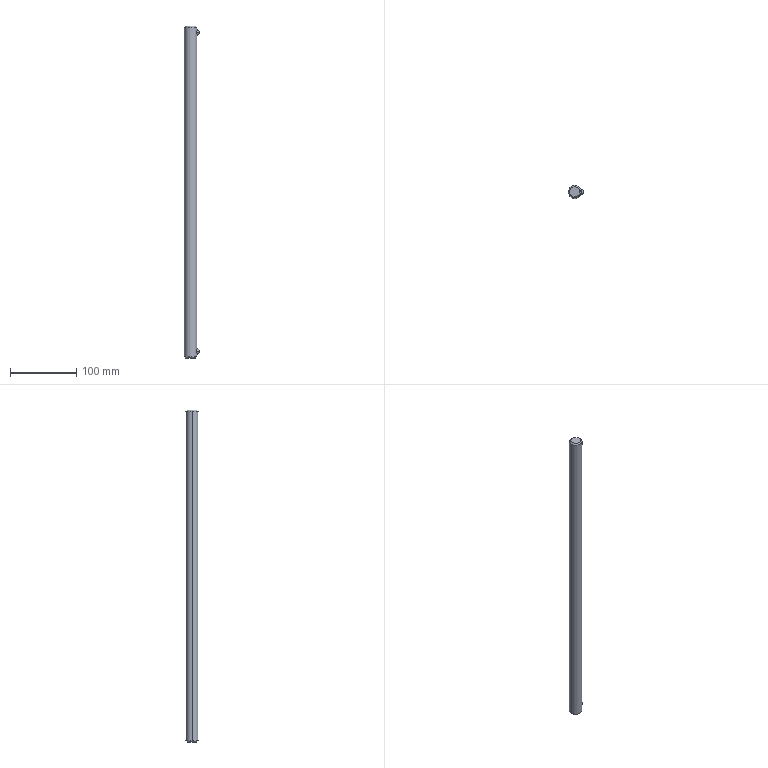Part | SolidWorks | features BaseBody 1 | 1 solid | 24 faces | box 23.05 x 19.05 x 500 mm | volume 142580 mm3 | spline 12 | cylinder 6 | cone 4 | plane 2 | commonest cylinder face diameters 8 x4 19.05 x2
STEP:
#1=CARTESIAN_POINT('',(22.554,-5.243,10.));
#2=VERTEX_POINT('',#1);
#3=CARTESIAN_POINT('',(18.554,-1.243,10.));
#4=VERTEX_POINT('',#3);
#5=CARTESIAN_POINT('',(18.554,-5.243,10.));
#6=DIRECTION('',(0.,0.,1.));
#7=DIRECTION('',(1.,0.,0.));
#8=AXIS2_PLACEMENT_3D('',#5,#6,#7);
#9=CIRCLE('',#8,4.);
#10=EDGE_CURVE('',#2,#4,#9,.T.);
#11=ORIENTED_EDGE('',*,*,#10,.F.);
#12=CARTESIAN_POINT('',(18.554,-9.243,10.));
#13=VERTEX_POINT('',#12);
#14=CARTESIAN_POINT('',(18.554,-5.243,10.));
#15=DIRECTION('',(0.,0.,-1.));
#16=DIRECTION('',(1.,0.,0.));
#17=AXIS2_PLACEMENT_3D('',#14,#15,#16);
#18=CIRCLE('',#17,4.);
#19=EDGE_CURVE('',#2,#13,#18,.T.);
#20=ORIENTED_EDGE('',*,*,#19,.T.);
#21=CARTESIAN_POINT('',(18.554,-8.022,7.123));
#22=VERTEX_POINT('',#21);
#23=CARTESIAN_POINT('',(18.554,-5.243,10.));
#24=DIRECTION('',(1.,0.,0.));
#25=DIRECTION('',(0.,1.,0.));
#26=AXIS2_PLACEMENT_3D('',#23,#24,#25);
#27=CIRCLE('',#26,4.);
#28=EDGE_CURVE('',#13,#22,#27,.T.);
#29=ORIENTED_EDGE('',*,*,#28,.T.);
#30=CARTESIAN_POINT('',(18.554,-2.464,7.123));
#31=VERTEX_POINT('',#30);
#32=CARTESIAN_POINT('',(18.554,-2.464,7.123));
#33=CARTESIAN_POINT('',(18.689,-2.875,6.725));
#34=CARTESIAN_POINT('',(18.951,-3.89,6.115));
#35=CARTESIAN_POINT('',(19.065,-6.011,5.891));
#36=CARTESIAN_POINT('',(18.757,-7.404,6.527));
#37=CARTESIAN_POINT('',(18.554,-8.022,7.123));
#38=B_SPLINE_CURVE_WITH_KNOTS('',3,(#32,#33,#34,#35,#36,#37),.UNSPECIFIED.,.F.,.F.,(4,1,1,4),(0.,0.2857,0.5714,1.),.UNSPECIFIED.);
#39=EDGE_CURVE('',#31,#22,#38,.T.);
#40=ORIENTED_EDGE('',*,*,#39,.F.);
#41=CARTESIAN_POINT('',(18.554,-5.243,10.));
#42=DIRECTION('',(1.,0.,0.));
#43=DIRECTION('',(0.,1.,0.));
#44=AXIS2_PLACEMENT_3D('',#41,#42,#43);
#45=CIRCLE('',#44,4.);
#46=EDGE_CURVE('',#31,#4,#45,.T.);
#47=ORIENTED_EDGE('',*,*,#46,.T.);
#48=EDGE_LOOP('',(#11,#20,#29,#40,#47));
#49=FACE_OUTER_BOUND('',#48,.T.);
#50=CARTESIAN_POINT('',(22.554,-5.243,10.));
#51=CARTESIAN_POINT('',(22.554,-5.243,10.));
#52=CARTESIAN_POINT('',(22.554,-5.243,10.));
#53=CARTESIAN_POINT('',(22.554,-5.243,10.));
#54=CARTESIAN_POINT('',(22.554,-7.586,10.));
#55=CARTESIAN_POINT('',(22.554,-7.586,5.314));
#56=CARTESIAN_POINT('',(22.554,-2.9,5.314));
#57=CARTESIAN_POINT('',(22.554,-2.9,10.));
#58=CARTESIAN_POINT('',(20.897,-9.243,10.));
#59=CARTESIAN_POINT('',(20.897,-9.243,2.));
#60=CARTESIAN_POINT('',(20.897,-1.243,2.));
#61=CARTESIAN_POINT('',(20.897,-1.243,10.));
#62=CARTESIAN_POINT('',(18.554,-9.243,10.));
#63=CARTESIAN_POINT('',(18.554,-9.243,2.));
#64=CARTESIAN_POINT('',(18.554,-1.243,2.));
#65=CARTESIAN_POINT('',(18.554,-1.243,10.));
#66=(BOUNDED_SURFACE()B_SPLINE_SURFACE(3,3,((#50,#51,#52,#53),(#54,#55,#56,#57),(#58,#59,#60,#61),(#62,#63,#64,#65)),.UNSPECIFIED.,.F.,.F.,.T.)B_SPLINE_SURFACE_WITH_KNOTS((4,4),(4,4),(0.,1.),(0.,1.),.UNSPECIFIED.)GEOMETRIC_REPRESENTATION_ITEM()RATIONAL_B_SPLINE_SURFACE(((1.,0.3333,0.3333,1.),(0.8047,0.2682,0.2682,0.8047),(0.8047,0.2682,0.2682,0.8047),(1.,0.3333,0.3333,1.)))REPRESENTATION_ITEM('')SURFACE());
#67=ADVANCED_FACE('',(#49),#66,.T.);
#68=CARTESIAN_POINT('',(22.554,-5.243,490.));
#69=VERTEX_POINT('',#68);
#70=CARTESIAN_POINT('',(18.554,-1.243,490.));
#71=VERTEX_POINT('',#70);
#72=CARTESIAN_POINT('',(18.554,-5.243,490.));
#73=DIRECTION('',(0.,0.,1.));
#74=DIRECTION('',(1.,0.,0.));
#75=AXIS2_PLACEMENT_3D('',#72,#73,#74);
#76=CIRCLE('',#75,4.);
#77=EDGE_CURVE('',#69,#71,#76,.T.);
#78=ORIENTED_EDGE('',*,*,#77,.F.);
#79=CARTESIAN_POINT('',(18.554,-9.243,490.));
#80=VERTEX_POINT('',#79);
#81=CARTESIAN_POINT('',(18.554,-5.243,490.));
#82=DIRECTION('',(0.,0.,-1.));
#83=DIRECTION('',(1.,0.,0.));
#84=AXIS2_PLACEMENT_3D('',#81,#82,#83);
#85=CIRCLE('',#84,4.);
#86=EDGE_CURVE('',#69,#80,#85,.T.);
#87=ORIENTED_EDGE('',*,*,#86,.T.);
#88=CARTESIAN_POINT('',(18.554,-8.022,487.123));
#89=VERTEX_POINT('',#88);
#90=CARTESIAN_POINT('',(18.554,-5.243,490.));
#91=DIRECTION('',(1.,0.,0.));
#92=DIRECTION('',(0.,1.,0.));
#93=AXIS2_PLACEMENT_3D('',#90,#91,#92);
#94=CIRCLE('',#93,4.);
#95=EDGE_CURVE('',#80,#89,#94,.T.);
#96=ORIENTED_EDGE('',*,*,#95,.T.);
#97=CARTESIAN_POINT('',(18.554,-2.464,487.123));
#98=VERTEX_POINT('',#97);
#99=CARTESIAN_POINT('',(18.554,-2.464,487.123));
#100=CARTESIAN_POINT('',(18.757,-3.081,486.527));
#101=CARTESIAN_POINT('',(19.067,-4.485,485.887));
#102=CARTESIAN_POINT('',(18.949,-6.602,486.119));
#103=CARTESIAN_POINT('',(18.689,-7.61,486.725));
#104=CARTESIAN_POINT('',(18.554,-8.022,487.123));
#105=B_SPLINE_CURVE_WITH_KNOTS('',3,(#99,#100,#101,#102,#103,#104),.UNSPECIFIED.,.F.,.F.,(4,1,1,4),(0.,0.4286,0.7143,1.),.UNSPECIFIED.);
#106=EDGE_CURVE('',#98,#89,#105,.T.);
#107=ORIENTED_EDGE('',*,*,#106,.F.);
#108=CARTESIAN_POINT('',(18.554,-5.243,490.));
#109=DIRECTION('',(1.,0.,0.));
#110=DIRECTION('',(0.,1.,0.));
#111=AXIS2_PLACEMENT_3D('',#108,#109,#110);
#112=CIRCLE('',#111,4.);
#113=EDGE_CURVE('',#98,#71,#112,.T.);
#114=ORIENTED_EDGE('',*,*,#113,.T.);
#115=EDGE_LOOP('',(#78,#87,#96,#107,#114));
#116=FACE_OUTER_BOUND('',#115,.T.);
#117=CARTESIAN_POINT('',(22.554,-5.243,490.));
#118=CARTESIAN_POINT('',(22.554,-5.243,490.));
#119=CARTESIAN_POINT('',(22.554,-5.243,490.));
#120=CARTESIAN_POINT('',(22.554,-5.243,490.));
#121=CARTESIAN_POINT('',(22.554,-7.586,490.));
#122=CARTESIAN_POINT('',(22.554,-7.586,485.314));
#123=CARTESIAN_POINT('',(22.554,-2.9,485.314));
#124=CARTESIAN_POINT('',(22.554,-2.9,490.));
#125=CARTESIAN_POINT('',(20.897,-9.243,490.));
#126=CARTESIAN_POINT('',(20.897,-9.243,482.));
#127=CARTESIAN_POINT('',(20.897,-1.243,482.));
#128=CARTESIAN_POINT('',(20.897,-1.243,490.));
#129=CARTESIAN_POINT('',(18.554,-9.243,490.));
#130=CARTESIAN_POINT('',(18.554,-9.243,482.));
#131=CARTESIAN_POINT('',(18.554,-1.243,482.));
#132=CARTESIAN_POINT('',(18.554,-1.243,490.));
#133=(BOUNDED_SURFACE()B_SPLINE_SURFACE(3,3,((#117,#118,#119,#120),(#121,#122,#123,#124),(#125,#126,#127,#128),(#129,#130,#131,#132)),.UNSPECIFIED.,.F.,.F.,.T.)B_SPLINE_SURFACE_WITH_KNOTS((4,4),(4,4),(0.,1.),(0.,1.),.UNSPECIFIED.)GEOMETRIC_REPRESENTATION_ITEM()RATIONAL_B_SPLINE_SURFACE(((1.,0.3333,0.3333,1.),(0.8047,0.2682,0.2682,0.8047),(0.8047,0.2682,0.2682,0.8047),(1.,0.3333,0.3333,1.)))REPRESENTATION_ITEM('')SURFACE());
#134=ADVANCED_FACE('',(#116),#133,.T.);
#135=CARTESIAN_POINT('',(18.554,-5.243,2.));
#136=VERTEX_POINT('',#135);
#137=CARTESIAN_POINT('',(-0.4959,-5.243,2.));
#138=VERTEX_POINT('',#137);
#139=CARTESIAN_POINT('',(9.029,-5.243,2.));
#140=DIRECTION('',(0.,0.,1.));
#141=DIRECTION('',(1.,0.,0.));
#142=AXIS2_PLACEMENT_3D('',#139,#140,#141);
#143=CIRCLE('',#142,9.525);
#144=EDGE_CURVE('',#136,#138,#143,.T.);
#145=ORIENTED_EDGE('',*,*,#144,.T.);
#146=CARTESIAN_POINT('',(-0.4959,-5.243,498.));
#147=VERTEX_POINT('',#146);
#148=CARTESIAN_POINT('',(-0.4959,-5.243,0.));
#149=DIRECTION('',(0.,0.,1.));
#150=VECTOR('',#149,1000.);
#151=LINE('',#148,#150);
#152=EDGE_CURVE('',#138,#147,#151,.T.);
#153=ORIENTED_EDGE('',*,*,#152,.T.);
#154=CARTESIAN_POINT('',(18.554,-5.243,498.));
#155=VERTEX_POINT('',#154);
#156=CARTESIAN_POINT('',(9.029,-5.243,498.));
#157=DIRECTION('',(0.,0.,-1.));
#158=DIRECTION('',(1.,0.,0.));
#159=AXIS2_PLACEMENT_3D('',#156,#157,#158);
#160=CIRCLE('',#159,9.525);
#161=EDGE_CURVE('',#147,#155,#160,.T.);
#162=ORIENTED_EDGE('',*,*,#161,.T.);
#163=CARTESIAN_POINT('',(18.554,-5.243,494.471));
#164=VERTEX_POINT('',#163);
#165=CARTESIAN_POINT('',(18.554,-5.243,0.));
#166=DIRECTION('',(0.,0.,1.));
#167=VECTOR('',#166,1000.);
#168=LINE('',#165,#167);
#169=EDGE_CURVE('',#164,#155,#168,.T.);
#170=ORIENTED_EDGE('',*,*,#169,.F.);
#171=CARTESIAN_POINT('',(18.079,-2.272,493.237));
#172=VERTEX_POINT('',#171);
#173=CARTESIAN_POINT('',(18.554,-5.243,494.471));
#174=CARTESIAN_POINT('',(18.554,-4.966,494.47));
#175=CARTESIAN_POINT('',(18.542,-4.689,494.443));
#176=CARTESIAN_POINT('',(18.494,-4.143,494.335));
#177=CARTESIAN_POINT('',(18.46,-3.88,494.255));
#178=CARTESIAN_POINT('',(18.372,-3.372,494.044));
#179=CARTESIAN_POINT('',(18.32,-3.131,493.915));
#180=CARTESIAN_POINT('',(18.205,-2.676,493.608));
#181=CARTESIAN_POINT('',(18.142,-2.465,493.432));
#182=CARTESIAN_POINT('',(18.079,-2.272,493.237));
#183=B_SPLINE_CURVE_WITH_KNOTS('',3,(#173,#174,#175,#176,#177,#178,#179,#180,#181,#182),.UNSPECIFIED.,.F.,.F.,(4,2,2,2,4),(0.4992,0.6244,0.7496,0.8748,1.),.UNSPECIFIED.);
#184=EDGE_CURVE('',#164,#172,#183,.T.);
#185=ORIENTED_EDGE('',*,*,#184,.T.);
#186=CARTESIAN_POINT('',(18.079,-2.272,486.763));
#187=VERTEX_POINT('',#186);
#188=CARTESIAN_POINT('',(18.079,-2.272,493.237));
#189=CARTESIAN_POINT('',(18.013,-2.069,493.03));
#190=CARTESIAN_POINT('',(17.946,-1.889,492.804));
#191=CARTESIAN_POINT('',(17.849,-1.645,492.429));
#192=CARTESIAN_POINT('',(17.818,-1.57,492.301));
#193=CARTESIAN_POINT('',(17.774,-1.467,492.104));
#194=CARTESIAN_POINT('',(17.753,-1.418,492.004));
#195=CARTESIAN_POINT('',(17.732,-1.372,491.902));
#196=CARTESIAN_POINT('',(17.719,-1.343,491.834));
#197=CARTESIAN_POINT('',(17.713,-1.329,491.801));
#198=CARTESIAN_POINT('',(17.653,-1.197,491.477));
#199=CARTESIAN_POINT('',(17.611,-1.111,491.185));
#200=CARTESIAN_POINT('',(17.555,-0.9959,490.595));
#201=CARTESIAN_POINT('',(17.541,-0.9679,490.299));
#202=CARTESIAN_POINT('',(17.542,-0.9692,489.843));
#203=CARTESIAN_POINT('',(17.545,-0.9767,489.692));
#204=CARTESIAN_POINT('',(17.56,-1.006,489.39));
#205=CARTESIAN_POINT('',(17.571,-1.029,489.237));
#206=CARTESIAN_POINT('',(17.6,-1.086,488.939));
#207=CARTESIAN_POINT('',(17.617,-1.122,488.793));
#208=CARTESIAN_POINT('',(17.647,-1.186,488.577));
#209=CARTESIAN_POINT('',(17.658,-1.209,488.506));
#210=CARTESIAN_POINT('',(17.681,-1.259,488.364));
#211=CARTESIAN_POINT('',(17.693,-1.286,488.293));
#212=CARTESIAN_POINT('',(17.731,-1.369,488.088));
#213=CARTESIAN_POINT('',(17.758,-1.431,487.955));
#214=CARTESIAN_POINT('',(17.802,-1.534,487.759));
#215=CARTESIAN_POINT('',(17.818,-1.57,487.694));
#216=CARTESIAN_POINT('',(17.849,-1.645,487.567));
#217=CARTESIAN_POINT('',(17.865,-1.685,487.502));
#218=CARTESIAN_POINT('',(17.945,-1.886,487.197));
#219=CARTESIAN_POINT('',(18.012,-2.068,486.971));
#220=CARTESIAN_POINT('',(18.079,-2.272,486.763));
#221=B_SPLINE_CURVE_WITH_KNOTS('',3,(#188,#189,#190,#191,#192,#193,#194,#195,#196,#197,#198,#199,#200,#201,#202,#203,#204,#205,#206,#207,#208,#209,#210,#211,#212,#213,#214,#215,#216,#217,#218,#219,#220),.UNSPECIFIED.,.F.,.F.,(4,2,2,1,2,2,2,2,2,2,2,2,2,2,2,2,4),(0.,0.125,0.1875,0.2187,0.2344,0.25,0.375,0.5,0.5625,0.625,0.6875,0.7187,0.75,0.8125,0.8437,0.875,1.),.UNSPECIFIED.);
#222=EDGE_CURVE('',#172,#187,#221,.T.);
#223=ORIENTED_EDGE('',*,*,#222,.T.);
#224=CARTESIAN_POINT('',(18.554,-5.243,485.529));
#225=VERTEX_POINT('',#224);
#226=CARTESIAN_POINT('',(18.079,-2.272,486.763));
#227=CARTESIAN_POINT('',(18.142,-2.463,486.569));
#228=CARTESIAN_POINT('',(18.204,-2.674,486.395));
#229=CARTESIAN_POINT('',(18.292,-3.02,486.163));
#230=CARTESIAN_POINT('',(18.319,-3.136,486.093));
#231=CARTESIAN_POINT('',(18.371,-3.378,485.964));
#232=CARTESIAN_POINT('',(18.395,-3.502,485.905));
#233=CARTESIAN_POINT('',(18.439,-3.758,485.799));
#234=CARTESIAN_POINT('',(18.459,-3.891,485.751));
#235=CARTESIAN_POINT('',(18.493,-4.155,485.67));
#236=CARTESIAN_POINT('',(18.507,-4.288,485.637));
#237=CARTESIAN_POINT('',(18.542,-4.692,485.556));
#238=CARTESIAN_POINT('',(18.554,-4.967,485.529));
#239=CARTESIAN_POINT('',(18.554,-5.243,485.529));
#240=B_SPLINE_CURVE_WITH_KNOTS('',3,(#226,#227,#228,#229,#230,#231,#232,#233,#234,#235,#236,#237,#238,#239),.UNSPECIFIED.,.F.,.F.,(4,2,2,2,2,2,4),(0.,0.1248,0.1872,0.2496,0.312,0.3744,0.4992),.UNSPECIFIED.);
#241=EDGE_CURVE('',#187,#225,#240,.T.);
#242=ORIENTED_EDGE('',*,*,#241,.T.);
#243=CARTESIAN_POINT('',(18.554,-5.243,14.471));
#244=VERTEX_POINT('',#243);
#245=CARTESIAN_POINT('',(18.554,-5.243,0.));
#246=DIRECTION('',(0.,0.,1.));
#247=VECTOR('',#246,1000.);
#248=LINE('',#245,#247);
#249=EDGE_CURVE('',#244,#225,#248,.T.);
#250=ORIENTED_EDGE('',*,*,#249,.F.);
#251=CARTESIAN_POINT('',(18.079,-2.272,13.237));
#252=VERTEX_POINT('',#251);
#253=CARTESIAN_POINT('',(18.554,-5.243,14.471));
#254=CARTESIAN_POINT('',(18.554,-5.105,14.471));
#255=CARTESIAN_POINT('',(18.551,-4.966,14.464));
#256=CARTESIAN_POINT('',(18.539,-4.69,14.437));
#257=CARTESIAN_POINT('',(18.53,-4.553,14.417));
#258=CARTESIAN_POINT('',(18.494,-4.143,14.335));
#259=CARTESIAN_POINT('',(18.46,-3.88,14.256));
#260=CARTESIAN_POINT('',(18.372,-3.372,14.045));
#261=CARTESIAN_POINT('',(18.32,-3.132,13.915));
#262=CARTESIAN_POINT('',(18.205,-2.676,13.608));
#263=CARTESIAN_POINT('',(18.142,-2.465,13.432));
#264=CARTESIAN_POINT('',(18.079,-2.272,13.237));
#265=B_SPLINE_CURVE_WITH_KNOTS('',3,(#253,#254,#255,#256,#257,#258,#259,#260,#261,#262,#263,#264),.UNSPECIFIED.,.F.,.F.,(4,2,2,2,2,4),(0.4992,0.5618,0.6244,0.7496,0.8748,1.),.UNSPECIFIED.);
#266=EDGE_CURVE('',#244,#252,#265,.T.);
#267=ORIENTED_EDGE('',*,*,#266,.T.);
#268=CARTESIAN_POINT('',(18.079,-2.272,6.763));
#269=VERTEX_POINT('',#268);
#270=CARTESIAN_POINT('',(18.079,-2.272,13.237));
#271=CARTESIAN_POINT('',(18.012,-2.069,13.03));
#272=CARTESIAN_POINT('',(17.946,-1.889,12.804));
#273=CARTESIAN_POINT('',(17.849,-1.645,12.43));
#274=CARTESIAN_POINT('',(17.818,-1.57,12.301));
#275=CARTESIAN_POINT('',(17.774,-1.467,12.104));
#276=CARTESIAN_POINT('',(17.753,-1.418,12.004));
#277=CARTESIAN_POINT('',(17.732,-1.372,11.902));
#278=CARTESIAN_POINT('',(17.719,-1.343,11.834));
#279=CARTESIAN_POINT('',(17.713,-1.329,11.801));
#280=CARTESIAN_POINT('',(17.653,-1.197,11.477));
#281=CARTESIAN_POINT('',(17.611,-1.11,11.186));
#282=CARTESIAN_POINT('',(17.555,-0.9955,10.596));
#283=CARTESIAN_POINT('',(17.541,-0.9675,10.299));
#284=CARTESIAN_POINT('',(17.541,-0.9687,9.844));
#285=CARTESIAN_POINT('',(17.545,-0.9763,9.693));
#286=CARTESIAN_POINT('',(17.56,-1.006,9.39));
#287=CARTESIAN_POINT('',(17.571,-1.028,9.238));
#288=CARTESIAN_POINT('',(17.599,-1.086,8.94));
#289=CARTESIAN_POINT('',(17.617,-1.122,8.794));
#290=CARTESIAN_POINT('',(17.647,-1.186,8.578));
#291=CARTESIAN_POINT('',(17.658,-1.209,8.506));
#292=CARTESIAN_POINT('',(17.681,-1.258,8.365));
#293=CARTESIAN_POINT('',(17.693,-1.285,8.293));
#294=CARTESIAN_POINT('',(17.731,-1.369,8.089));
#295=CARTESIAN_POINT('',(17.758,-1.431,7.955));
#296=CARTESIAN_POINT('',(17.802,-1.534,7.759));
#297=CARTESIAN_POINT('',(17.817,-1.57,7.695));
#298=CARTESIAN_POINT('',(17.849,-1.645,7.567));
#299=CARTESIAN_POINT('',(17.865,-1.685,7.503));
#300=CARTESIAN_POINT('',(17.945,-1.886,7.197));
#301=CARTESIAN_POINT('',(18.012,-2.068,6.971));
#302=CARTESIAN_POINT('',(18.079,-2.272,6.763));
#303=B_SPLINE_CURVE_WITH_KNOTS('',3,(#270,#271,#272,#273,#274,#275,#276,#277,#278,#279,#280,#281,#282,#283,#284,#285,#286,#287,#288,#289,#290,#291,#292,#293,#294,#295,#296,#297,#298,#299,#300,#301,#302),.UNSPECIFIED.,.F.,.F.,(4,2,2,1,2,2,2,2,2,2,2,2,2,2,2,2,4),(0.,0.125,0.1875,0.2187,0.2344,0.25,0.375,0.5,0.5625,0.625,0.6875,0.7187,0.75,0.8125,0.8437,0.875,1.),.UNSPECIFIED.);
#304=EDGE_CURVE('',#252,#269,#303,.T.);
#305=ORIENTED_EDGE('',*,*,#304,.T.);
#306=CARTESIAN_POINT('',(18.554,-5.243,5.53));
#307=VERTEX_POINT('',#306);
#308=CARTESIAN_POINT('',(18.079,-2.272,6.763));
#309=CARTESIAN_POINT('',(18.205,-2.656,6.373));
#310=CARTESIAN_POINT('',(18.329,-3.119,6.061));
#311=CARTESIAN_POINT('',(18.46,-3.881,5.744));
#312=CARTESIAN_POINT('',(18.495,-4.145,5.664));
#313=CARTESIAN_POINT('',(18.53,-4.554,5.584));
#314=CARTESIAN_POINT('',(18.539,-4.691,5.563));
#315=CARTESIAN_POINT('',(18.551,-4.966,5.537));
#316=CARTESIAN_POINT('',(18.554,-5.105,5.53));
#317=CARTESIAN_POINT('',(18.554,-5.243,5.53));
#318=B_SPLINE_CURVE_WITH_KNOTS('',3,(#308,#309,#310,#311,#312,#313,#314,#315,#316,#317),.UNSPECIFIED.,.F.,.F.,(4,2,2,2,4),(0.,0.2497,0.3746,0.437,0.4995),.UNSPECIFIED.);
#319=EDGE_CURVE('',#269,#307,#318,.T.);
#320=ORIENTED_EDGE('',*,*,#319,.T.);
#321=CARTESIAN_POINT('',(18.554,-5.243,0.));
#322=DIRECTION('',(0.,0.,1.));
#323=VECTOR('',#322,1000.);
#324=LINE('',#321,#323);
#325=EDGE_CURVE('',#136,#307,#324,.T.);
#326=ORIENTED_EDGE('',*,*,#325,.F.);
#327=EDGE_LOOP('',(#145,#153,#162,#170,#185,#223,#242,#250,#267,#305,#320,#326));
#328=FACE_OUTER_BOUND('',#327,.T.);
#329=CARTESIAN_POINT('',(9.029,-5.243,0.));
#330=DIRECTION('',(0.,0.,1.));
#331=DIRECTION('',(1.,0.,0.));
#332=AXIS2_PLACEMENT_3D('',#329,#330,#331);
#333=CYLINDRICAL_SURFACE('',#332,9.525);
#334=ADVANCED_FACE('',(#328),#333,.T.);
#335=CARTESIAN_POINT('',(1.504,-5.243,500.));
#336=VERTEX_POINT('',#335);
#337=CARTESIAN_POINT('',(16.554,-5.243,500.));
#338=VERTEX_POINT('',#337);
#339=CARTESIAN_POINT('',(9.029,-5.243,500.));
#340=DIRECTION('',(0.,0.,-1.));
#341=DIRECTION('',(-1.,0.,0.));
#342=AXIS2_PLACEMENT_3D('',#339,#340,#341);
#343=CIRCLE('',#342,7.525);
#344=EDGE_CURVE('',#336,#338,#343,.T.);
#345=ORIENTED_EDGE('',*,*,#344,.T.);
#346=CARTESIAN_POINT('',(18.554,-5.243,498.));
#347=DIRECTION('',(0.7071,0.,-0.7071));
#348=VECTOR('',#347,1000.);
#349=LINE('',#346,#348);
#350=EDGE_CURVE('',#338,#155,#349,.T.);
#351=ORIENTED_EDGE('',*,*,#350,.T.);
#352=ORIENTED_EDGE('',*,*,#161,.F.);
#353=CARTESIAN_POINT('',(-0.4959,-5.243,498.));
#354=DIRECTION('',(-0.7071,0.,-0.7071));
#355=VECTOR('',#354,1000.);
#356=LINE('',#353,#355);
#357=EDGE_CURVE('',#336,#147,#356,.T.);
#358=ORIENTED_EDGE('',*,*,#357,.F.);
#359=EDGE_LOOP('',(#345,#351,#352,#358));
#360=FACE_OUTER_BOUND('',#359,.T.);
#361=CARTESIAN_POINT('',(9.029,-5.243,498.));
#362=DIRECTION('',(0.,0.,-1.));
#363=DIRECTION('',(-1.,0.,0.));
#364=AXIS2_PLACEMENT_3D('',#361,#362,#363);
#365=CONICAL_SURFACE('',#364,9.525,0.7854);
#366=ADVANCED_FACE('',(#360),#365,.T.);
#367=CARTESIAN_POINT('',(16.554,-5.243,0.));
#368=VERTEX_POINT('',#367);
#369=CARTESIAN_POINT('',(1.504,-5.243,0.));
#370=VERTEX_POINT('',#369);
#371=CARTESIAN_POINT('',(9.029,-5.243,0.));
#372=DIRECTION('',(0.,0.,1.));
#373=DIRECTION('',(1.,0.,0.));
#374=AXIS2_PLACEMENT_3D('',#371,#372,#373);
#375=CIRCLE('',#374,7.525);
#376=EDGE_CURVE('',#368,#370,#375,.T.);
#377=ORIENTED_EDGE('',*,*,#376,.T.);
#378=CARTESIAN_POINT('',(-0.4959,-5.243,2.));
#379=DIRECTION('',(-0.7071,0.,0.7071));
#380=VECTOR('',#379,1000.);
#381=LINE('',#378,#380);
#382=EDGE_CURVE('',#370,#138,#381,.T.);
#383=ORIENTED_EDGE('',*,*,#382,.T.);
#384=ORIENTED_EDGE('',*,*,#144,.F.);
#385=CARTESIAN_POINT('',(18.554,-5.243,2.));
#386=DIRECTION('',(0.7071,0.,0.7071));
#387=VECTOR('',#386,1000.);
#388=LINE('',#385,#387);
#389=EDGE_CURVE('',#368,#136,#388,.T.);
#390=ORIENTED_EDGE('',*,*,#389,.F.);
#391=EDGE_LOOP('',(#377,#383,#384,#390));
#392=FACE_OUTER_BOUND('',#391,.T.);
#393=CARTESIAN_POINT('',(9.029,-5.243,2.));
#394=DIRECTION('',(0.,0.,1.));
#395=DIRECTION('',(1.,0.,0.));
#396=AXIS2_PLACEMENT_3D('',#393,#394,#395);
#397=CONICAL_SURFACE('',#396,9.525,0.7854);
#398=ADVANCED_FACE('',(#392),#397,.T.);
#399=ORIENTED_EDGE('',*,*,#152,.F.);
#400=CARTESIAN_POINT('',(9.029,-5.243,2.));
#401=DIRECTION('',(0.,0.,1.));
#402=DIRECTION('',(1.,0.,0.));
#403=AXIS2_PLACEMENT_3D('',#400,#401,#402);
#404=CIRCLE('',#403,9.525);
#405=EDGE_CURVE('',#138,#136,#404,.T.);
#406=ORIENTED_EDGE('',*,*,#405,.T.);
#407=ORIENTED_EDGE('',*,*,#325,.T.);
#408=CARTESIAN_POINT('',(18.079,-8.213,6.763));
#409=VERTEX_POINT('',#408);
#410=CARTESIAN_POINT('',(18.554,-5.243,5.53));
#411=CARTESIAN_POINT('',(18.554,-5.519,5.529));
#412=CARTESIAN_POINT('',(18.542,-5.795,5.556));
#413=CARTESIAN_POINT('',(18.495,-6.333,5.663));
#414=CARTESIAN_POINT('',(18.461,-6.597,5.744));
#415=CARTESIAN_POINT('',(18.394,-6.985,5.905));
#416=CARTESIAN_POINT('',(18.371,-7.108,5.963));
#417=CARTESIAN_POINT('',(18.319,-7.349,6.093));
#418=CARTESIAN_POINT('',(18.292,-7.467,6.163));
#419=CARTESIAN_POINT('',(18.234,-7.695,6.316));
#420=CARTESIAN_POINT('',(18.203,-7.806,6.399));
#421=CARTESIAN_POINT('',(18.142,-8.017,6.574));
#422=CARTESIAN_POINT('',(18.111,-8.117,6.666));
#423=CARTESIAN_POINT('',(18.079,-8.213,6.763));
#424=B_SPLINE_CURVE_WITH_KNOTS('',3,(#410,#411,#412,#413,#414,#415,#416,#417,#418,#419,#420,#421,#422,#423),.UNSPECIFIED.,.F.,.F.,(4,2,2,2,2,2,4),(0.4995,0.6246,0.7497,0.8123,0.8749,0.9374,1.),.UNSPECIFIED.);
#425=EDGE_CURVE('',#307,#409,#424,.T.);
#426=ORIENTED_EDGE('',*,*,#425,.T.);
#427=CARTESIAN_POINT('',(18.079,-8.213,13.237));
#428=VERTEX_POINT('',#427);
#429=CARTESIAN_POINT('',(18.079,-8.213,6.763));
#430=CARTESIAN_POINT('',(18.012,-8.416,6.97));
#431=CARTESIAN_POINT('',(17.946,-8.597,7.196));
#432=CARTESIAN_POINT('',(17.849,-8.841,7.57));
#433=CARTESIAN_POINT('',(17.818,-8.916,7.699));
#434=CARTESIAN_POINT('',(17.774,-9.019,7.896));
#435=CARTESIAN_POINT('',(17.753,-9.068,7.996));
#436=CARTESIAN_POINT('',(17.732,-9.113,8.098));
#437=CARTESIAN_POINT('',(17.719,-9.143,8.166));
#438=CARTESIAN_POINT('',(17.713,-9.157,8.199));
#439=CARTESIAN_POINT('',(17.653,-9.289,8.523));
#440=CARTESIAN_POINT('',(17.611,-9.375,8.814));
#441=CARTESIAN_POINT('',(17.555,-9.49,9.404));
#442=CARTESIAN_POINT('',(17.541,-9.518,9.701));
#443=CARTESIAN_POINT('',(17.541,-9.517,10.156));
#444=CARTESIAN_POINT('',(17.545,-9.509,10.307));
#445=CARTESIAN_POINT('',(17.56,-9.479,10.61));
#446=CARTESIAN_POINT('',(17.571,-9.457,10.762));
#447=CARTESIAN_POINT('',(17.599,-9.399,11.06));
#448=CARTESIAN_POINT('',(17.617,-9.364,11.207));
#449=CARTESIAN_POINT('',(17.647,-9.3,11.423));
#450=CARTESIAN_POINT('',(17.658,-9.277,11.494));
#451=CARTESIAN_POINT('',(17.681,-9.227,11.635));
#452=CARTESIAN_POINT('',(17.693,-9.2,11.707));
#453=CARTESIAN_POINT('',(17.731,-9.117,11.911));
#454=CARTESIAN_POINT('',(17.758,-9.055,12.045));
#455=CARTESIAN_POINT('',(17.802,-8.952,12.241));
#456=CARTESIAN_POINT('',(17.818,-8.916,12.305));
#457=CARTESIAN_POINT('',(17.849,-8.841,12.433));
#458=CARTESIAN_POINT('',(17.865,-8.8,12.498));
#459=CARTESIAN_POINT('',(17.945,-8.6,12.803));
#460=CARTESIAN_POINT('',(18.012,-8.418,13.029));
#461=CARTESIAN_POINT('',(18.079,-8.213,13.237));
#462=B_SPLINE_CURVE_WITH_KNOTS('',3,(#429,#430,#431,#432,#433,#434,#435,#436,#437,#438,#439,#440,#441,#442,#443,#444,#445,#446,#447,#448,#449,#450,#451,#452,#453,#454,#455,#456,#457,#458,#459,#460,#461),.UNSPECIFIED.,.F.,.F.,(4,2,2,1,2,2,2,2,2,2,2,2,2,2,2,2,4),(0.,0.125,0.1875,0.2188,0.2344,0.25,0.375,0.5,0.5625,0.625,0.6875,0.7187,0.75,0.8125,0.8437,0.875,1.),.UNSPECIFIED.);
#463=EDGE_CURVE('',#409,#428,#462,.T.);
#464=ORIENTED_EDGE('',*,*,#463,.T.);
#465=CARTESIAN_POINT('',(18.079,-8.213,13.237));
#466=CARTESIAN_POINT('',(18.142,-8.022,13.431));
#467=CARTESIAN_POINT('',(18.204,-7.812,13.605));
#468=CARTESIAN_POINT('',(18.292,-7.466,13.837));
#469=CARTESIAN_POINT('',(18.319,-7.349,13.907));
#470=CARTESIAN_POINT('',(18.371,-7.108,14.036));
#471=CARTESIAN_POINT('',(18.395,-6.983,14.095));
#472=CARTESIAN_POINT('',(18.439,-6.728,14.202));
#473=CARTESIAN_POINT('',(18.459,-6.595,14.249));
#474=CARTESIAN_POINT('',(18.493,-6.331,14.33));
#475=CARTESIAN_POINT('',(18.522,-6.064,14.397));
#476=CARTESIAN_POINT('',(18.539,-5.792,14.438));
#477=CARTESIAN_POINT('',(18.551,-5.519,14.464));
#478=CARTESIAN_POINT('',(18.554,-5.38,14.471));
#479=CARTESIAN_POINT('',(18.554,-5.243,14.471));
#480=B_SPLINE_CURVE_WITH_KNOTS('',3,(#465,#466,#467,#468,#469,#470,#471,#472,#473,#474,#475,#476,#477,#478,#479),.UNSPECIFIED.,.F.,.F.,(4,2,2,2,2,1,2,4),(0.,0.1248,0.1872,0.2496,0.312,0.3744,0.4368,0.4992),.UNSPECIFIED.);
#481=EDGE_CURVE('',#428,#244,#480,.T.);
#482=ORIENTED_EDGE('',*,*,#481,.T.);
#483=ORIENTED_EDGE('',*,*,#249,.T.);
#484=CARTESIAN_POINT('',(18.079,-8.213,486.763));
#485=VERTEX_POINT('',#484);
#486=CARTESIAN_POINT('',(18.554,-5.243,485.529));
#487=CARTESIAN_POINT('',(18.554,-5.519,485.53));
#488=CARTESIAN_POINT('',(18.542,-5.796,485.557));
#489=CARTESIAN_POINT('',(18.494,-6.342,485.665));
#490=CARTESIAN_POINT('',(18.46,-6.605,485.745));
#491=CARTESIAN_POINT('',(18.372,-7.113,485.956));
#492=CARTESIAN_POINT('',(18.32,-7.354,486.085));
#493=CARTESIAN_POINT('',(18.205,-7.81,486.392));
#494=CARTESIAN_POINT('',(18.142,-8.021,486.568));
#495=CARTESIAN_POINT('',(18.079,-8.213,486.763));
#496=B_SPLINE_CURVE_WITH_KNOTS('',3,(#486,#487,#488,#489,#490,#491,#492,#493,#494,#495),.UNSPECIFIED.,.F.,.F.,(4,2,2,2,4),(0.4992,0.6244,0.7496,0.8748,1.),.UNSPECIFIED.);
#497=EDGE_CURVE('',#225,#485,#496,.T.);
#498=ORIENTED_EDGE('',*,*,#497,.T.);
#499=CARTESIAN_POINT('',(18.079,-8.213,493.237));
#500=VERTEX_POINT('',#499);
#501=CARTESIAN_POINT('',(18.079,-8.213,486.763));
#502=CARTESIAN_POINT('',(18.013,-8.416,486.97));
#503=CARTESIAN_POINT('',(17.946,-8.597,487.196));
#504=CARTESIAN_POINT('',(17.849,-8.841,487.571));
#505=CARTESIAN_POINT('',(17.818,-8.915,487.699));
#506=CARTESIAN_POINT('',(17.774,-9.018,487.896));
#507=CARTESIAN_POINT('',(17.753,-9.067,487.996));
#508=CARTESIAN_POINT('',(17.732,-9.113,488.098));
#509=CARTESIAN_POINT('',(17.719,-9.143,488.166));
#510=CARTESIAN_POINT('',(17.713,-9.157,488.199));
#511=CARTESIAN_POINT('',(17.653,-9.288,488.523));
#512=CARTESIAN_POINT('',(17.611,-9.375,488.815));
#513=CARTESIAN_POINT('',(17.555,-9.49,489.405));
#514=CARTESIAN_POINT('',(17.541,-9.518,489.701));
#515=CARTESIAN_POINT('',(17.542,-9.516,490.157));
#516=CARTESIAN_POINT('',(17.545,-9.509,490.308));
#517=CARTESIAN_POINT('',(17.56,-9.479,490.61));
#518=CARTESIAN_POINT('',(17.571,-9.457,490.763));
#519=CARTESIAN_POINT('',(17.6,-9.399,491.061));
#520=CARTESIAN_POINT('',(17.617,-9.363,491.207));
#521=CARTESIAN_POINT('',(17.647,-9.299,491.423));
#522=CARTESIAN_POINT('',(17.658,-9.276,491.494));
#523=CARTESIAN_POINT('',(17.681,-9.227,491.636));
#524=CARTESIAN_POINT('',(17.693,-9.2,491.707));
#525=CARTESIAN_POINT('',(17.731,-9.117,491.912));
#526=CARTESIAN_POINT('',(17.758,-9.055,492.045));
#527=CARTESIAN_POINT('',(17.802,-8.952,492.241));
#528=CARTESIAN_POINT('',(17.818,-8.916,492.306));
#529=CARTESIAN_POINT('',(17.849,-8.84,492.433));
#530=CARTESIAN_POINT('',(17.865,-8.8,492.498));
#531=CARTESIAN_POINT('',(17.945,-8.6,492.803));
#532=CARTESIAN_POINT('',(18.012,-8.418,493.029));
#533=CARTESIAN_POINT('',(18.079,-8.213,493.237));
#534=B_SPLINE_CURVE_WITH_KNOTS('',3,(#501,#502,#503,#504,#505,#506,#507,#508,#509,#510,#511,#512,#513,#514,#515,#516,#517,#518,#519,#520,#521,#522,#523,#524,#525,#526,#527,#528,#529,#530,#531,#532,#533),.UNSPECIFIED.,.F.,.F.,(4,2,2,1,2,2,2,2,2,2,2,2,2,2,2,2,4),(0.,0.125,0.1875,0.2188,0.2344,0.25,0.375,0.5,0.5625,0.625,0.6875,0.7188,0.75,0.8125,0.8438,0.875,1.),.UNSPECIFIED.);
#535=EDGE_CURVE('',#485,#500,#534,.T.);
#536=ORIENTED_EDGE('',*,*,#535,.T.);
#537=CARTESIAN_POINT('',(18.079,-8.213,493.237));
#538=CARTESIAN_POINT('',(18.142,-8.022,493.431));
#539=CARTESIAN_POINT('',(18.204,-7.812,493.605));
#540=CARTESIAN_POINT('',(18.292,-7.466,493.837));
#541=CARTESIAN_POINT('',(18.319,-7.349,493.907));
#542=CARTESIAN_POINT('',(18.371,-7.108,494.036));
#543=CARTESIAN_POINT('',(18.395,-6.983,494.095));
#544=CARTESIAN_POINT('',(18.439,-6.728,494.201));
#545=CARTESIAN_POINT('',(18.459,-6.595,494.249));
#546=CARTESIAN_POINT('',(18.493,-6.331,494.33));
#547=CARTESIAN_POINT('',(18.507,-6.197,494.363));
#548=CARTESIAN_POINT('',(18.542,-5.794,494.444));
#549=CARTESIAN_POINT('',(18.554,-5.518,494.471));
#550=CARTESIAN_POINT('',(18.554,-5.243,494.471));
#551=B_SPLINE_CURVE_WITH_KNOTS('',3,(#537,#538,#539,#540,#541,#542,#543,#544,#545,#546,#547,#548,#549,#550),.UNSPECIFIED.,.F.,.F.,(4,2,2,2,2,2,4),(0.,0.1248,0.1872,0.2496,0.312,0.3744,0.4992),.UNSPECIFIED.);
#552=EDGE_CURVE('',#500,#164,#551,.T.);
#553=ORIENTED_EDGE('',*,*,#552,.T.);
#554=ORIENTED_EDGE('',*,*,#169,.T.);
#555=CARTESIAN_POINT('',(9.029,-5.243,498.));
#556=DIRECTION('',(0.,0.,-1.));
#557=DIRECTION('',(1.,0.,0.));
#558=AXIS2_PLACEMENT_3D('',#555,#556,#557);
#559=CIRCLE('',#558,9.525);
#560=EDGE_CURVE('',#155,#147,#559,.T.);
#561=ORIENTED_EDGE('',*,*,#560,.T.);
#562=EDGE_LOOP('',(#399,#406,#407,#426,#464,#482,#483,#498,#536,#553,#554,#561));
#563=FACE_OUTER_BOUND('',#562,.T.);
#564=CARTESIAN_POINT('',(9.029,-5.243,0.));
#565=DIRECTION('',(0.,0.,1.));
#566=DIRECTION('',(1.,0.,0.));
#567=AXIS2_PLACEMENT_3D('',#564,#565,#566);
#568=CYLINDRICAL_SURFACE('',#567,9.525);
#569=ADVANCED_FACE('',(#563),#568,.T.);
#570=CARTESIAN_POINT('',(18.554,-8.022,12.877));
#571=VERTEX_POINT('',#570);
#572=CARTESIAN_POINT('',(18.079,-8.213,13.237));
#573=CARTESIAN_POINT('',(18.103,-8.141,13.153));
#574=CARTESIAN_POINT('',(18.226,-8.021,12.988));
#575=CARTESIAN_POINT('',(18.444,-8.003,12.895));
#576=CARTESIAN_POINT('',(18.554,-8.022,12.877));
#577=B_SPLINE_CURVE_WITH_KNOTS('',3,(#572,#573,#574,#575,#576),.UNSPECIFIED.,.F.,.F.,(4,1,4),(0.,0.5,1.),.UNSPECIFIED.);
#578=EDGE_CURVE('',#428,#571,#577,.T.);
#579=ORIENTED_EDGE('',*,*,#578,.T.);
#580=CARTESIAN_POINT('',(18.554,-2.464,12.877));
#581=VERTEX_POINT('',#580);
#582=CARTESIAN_POINT('',(18.554,-8.022,12.877));
#583=CARTESIAN_POINT('',(18.757,-7.404,13.473));
#584=CARTESIAN_POINT('',(19.067,-6.001,14.113));
#585=CARTESIAN_POINT('',(18.95,-3.883,13.882));
#586=CARTESIAN_POINT('',(18.689,-2.875,13.275));
#587=CARTESIAN_POINT('',(18.554,-2.464,12.877));
#588=B_SPLINE_CURVE_WITH_KNOTS('',3,(#582,#583,#584,#585,#586,#587),.UNSPECIFIED.,.F.,.F.,(4,1,1,4),(0.,0.4286,0.7143,1.),.UNSPECIFIED.);
#589=EDGE_CURVE('',#571,#581,#588,.T.);
#590=ORIENTED_EDGE('',*,*,#589,.T.);
#591=CARTESIAN_POINT('',(18.554,-2.464,12.877));
#592=CARTESIAN_POINT('',(18.444,-2.482,12.895));
#593=CARTESIAN_POINT('',(18.226,-2.464,12.988));
#594=CARTESIAN_POINT('',(18.103,-2.345,13.153));
#595=CARTESIAN_POINT('',(18.079,-2.272,13.237));
#596=B_SPLINE_CURVE_WITH_KNOTS('',3,(#591,#592,#593,#594,#595),.UNSPECIFIED.,.F.,.F.,(4,1,4),(0.,0.5,1.),.UNSPECIFIED.);
#597=EDGE_CURVE('',#581,#252,#596,.T.);
#598=ORIENTED_EDGE('',*,*,#597,.T.);
#599=ORIENTED_EDGE('',*,*,#266,.F.);
#600=ORIENTED_EDGE('',*,*,#481,.F.);
#601=EDGE_LOOP('',(#579,#590,#598,#599,#600));
#602=FACE_OUTER_BOUND('',#601,.T.);
#603=CARTESIAN_POINT('',(18.079,-8.213,13.237));
#604=CARTESIAN_POINT('',(18.296,-7.553,13.908));
#605=CARTESIAN_POINT('',(18.627,-6.053,14.627));
#606=CARTESIAN_POINT('',(18.502,-3.79,14.367));
#607=CARTESIAN_POINT('',(18.224,-2.712,13.684));
#608=CARTESIAN_POINT('',(18.079,-2.272,13.237));
#609=CARTESIAN_POINT('',(18.103,-8.141,13.153));
#610=CARTESIAN_POINT('',(18.309,-7.493,13.805));
#611=CARTESIAN_POINT('',(18.623,-6.03,14.5));
#612=CARTESIAN_POINT('',(18.505,-3.83,14.249));
#613=CARTESIAN_POINT('',(18.241,-2.776,13.588));
#614=CARTESIAN_POINT('',(18.103,-2.345,13.153));
#615=CARTESIAN_POINT('',(18.226,-8.021,12.988));
#616=CARTESIAN_POINT('',(18.42,-7.395,13.601));
#617=CARTESIAN_POINT('',(18.711,-5.993,14.247));
#618=CARTESIAN_POINT('',(18.601,-3.896,14.014));
#619=CARTESIAN_POINT('',(18.355,-2.882,13.397));
#620=CARTESIAN_POINT('',(18.226,-2.464,12.988));
#621=CARTESIAN_POINT('',(18.444,-8.003,12.895));
#622=CARTESIAN_POINT('',(18.643,-7.386,13.491));
#623=CARTESIAN_POINT('',(18.944,-5.991,14.125));
#624=CARTESIAN_POINT('',(18.83,-3.899,13.896));
#625=CARTESIAN_POINT('',(18.577,-2.894,13.293));
#626=CARTESIAN_POINT('',(18.444,-2.482,12.895));
#627=CARTESIAN_POINT('',(18.554,-8.022,12.877));
#628=CARTESIAN_POINT('',(18.757,-7.404,13.473));
#629=CARTESIAN_POINT('',(19.067,-6.001,14.113));
#630=CARTESIAN_POINT('',(18.95,-3.883,13.882));
#631=CARTESIAN_POINT('',(18.689,-2.875,13.275));
#632=CARTESIAN_POINT('',(18.554,-2.464,12.877));
#633=B_SPLINE_SURFACE_WITH_KNOTS('',3,3,((#603,#604,#605,#606,#607,#608),(#609,#610,#611,#612,#613,#614),(#615,#616,#617,#618,#619,#620),(#621,#622,#623,#624,#625,#626),(#627,#628,#629,#630,#631,#632)),.UNSPECIFIED.,.F.,.F.,.F.,(4,1,4),(4,1,1,4),(0.,0.5,1.),(-0.6947,-0.397,-0.1985,0.),.UNSPECIFIED.);
#634=ADVANCED_FACE('',(#602),#633,.T.);
#635=CARTESIAN_POINT('',(18.079,-8.213,6.763));
#636=CARTESIAN_POINT('',(18.103,-8.141,6.847));
#637=CARTESIAN_POINT('',(18.226,-8.021,7.012));
#638=CARTESIAN_POINT('',(18.444,-8.003,7.105));
#639=CARTESIAN_POINT('',(18.554,-8.022,7.123));
#640=B_SPLINE_CURVE_WITH_KNOTS('',3,(#635,#636,#637,#638,#639),.UNSPECIFIED.,.F.,.F.,(4,1,4),(0.,0.5,1.),.UNSPECIFIED.);
#641=EDGE_CURVE('',#409,#22,#640,.T.);
#642=ORIENTED_EDGE('',*,*,#641,.T.);
#643=CARTESIAN_POINT('',(18.554,-8.022,7.123));
#644=CARTESIAN_POINT('',(18.314,-8.671,7.75));
#645=CARTESIAN_POINT('',(17.892,-9.401,9.203));
#646=CARTESIAN_POINT('',(18.056,-9.135,11.422));
#647=CARTESIAN_POINT('',(18.394,-8.455,12.459));
#648=CARTESIAN_POINT('',(18.554,-8.022,12.877));
#649=B_SPLINE_CURVE_WITH_KNOTS('',3,(#643,#644,#645,#646,#647,#648),.UNSPECIFIED.,.F.,.F.,(4,1,1,4),(0.,0.4286,0.7143,1.),.UNSPECIFIED.);
#650=EDGE_CURVE('',#22,#571,#649,.T.);
#651=ORIENTED_EDGE('',*,*,#650,.T.);
#652=ORIENTED_EDGE('',*,*,#578,.F.);
#653=ORIENTED_EDGE('',*,*,#463,.F.);
#654=EDGE_LOOP('',(#642,#651,#652,#653));
#655=FACE_OUTER_BOUND('',#654,.T.);
#656=CARTESIAN_POINT('',(18.079,-8.213,6.763));
#657=CARTESIAN_POINT('',(17.851,-8.907,7.469));
#658=CARTESIAN_POINT('',(17.45,-9.687,9.104));
#659=CARTESIAN_POINT('',(17.606,-9.403,11.6));
#660=CARTESIAN_POINT('',(17.927,-8.676,12.766));
#661=CARTESIAN_POINT('',(18.079,-8.213,13.237));
#662=CARTESIAN_POINT('',(18.103,-8.141,6.847));
#663=CARTESIAN_POINT('',(17.885,-8.825,7.529));
#664=CARTESIAN_POINT('',(17.494,-9.605,9.123));
#665=CARTESIAN_POINT('',(17.646,-9.32,11.564));
#666=CARTESIAN_POINT('',(17.957,-8.597,12.698));
#667=CARTESIAN_POINT('',(18.103,-8.141,13.153));
#668=CARTESIAN_POINT('',(18.226,-8.021,7.012));
#669=CARTESIAN_POINT('',(18.012,-8.689,7.65));
#670=CARTESIAN_POINT('',(17.623,-9.463,9.162));
#671=CARTESIAN_POINT('',(17.774,-9.18,11.493));
#672=CARTESIAN_POINT('',(18.083,-8.466,12.562));
#673=CARTESIAN_POINT('',(18.226,-8.021,12.988));
#674=CARTESIAN_POINT('',(18.444,-8.003,7.105));
#675=CARTESIAN_POINT('',(18.213,-8.657,7.728));
#676=CARTESIAN_POINT('',(17.803,-9.405,9.192));
#677=CARTESIAN_POINT('',(17.962,-9.132,11.44));
#678=CARTESIAN_POINT('',(18.29,-8.439,12.479));
#679=CARTESIAN_POINT('',(18.444,-8.003,12.895));
#680=CARTESIAN_POINT('',(18.554,-8.022,7.123));
#681=CARTESIAN_POINT('',(18.314,-8.671,7.75));
#682=CARTESIAN_POINT('',(17.892,-9.401,9.203));
#683=CARTESIAN_POINT('',(18.056,-9.135,11.422));
#684=CARTESIAN_POINT('',(18.394,-8.455,12.459));
#685=CARTESIAN_POINT('',(18.554,-8.022,12.877));
#686=B_SPLINE_SURFACE_WITH_KNOTS('',3,3,((#656,#657,#658,#659,#660,#661),(#662,#663,#664,#665,#666,#667),(#668,#669,#670,#671,#672,#673),(#674,#675,#676,#677,#678,#679),(#680,#681,#682,#683,#684,#685)),.UNSPECIFIED.,.F.,.F.,.F.,(4,1,4),(4,1,1,4),(0.,0.5,1.),(0.,0.313,0.5216,0.7303),.UNSPECIFIED.);
#687=ADVANCED_FACE('',(#655),#686,.T.);
#688=CARTESIAN_POINT('',(18.079,-2.272,6.763));
#689=CARTESIAN_POINT('',(18.103,-2.345,6.847));
#690=CARTESIAN_POINT('',(18.226,-2.464,7.012));
#691=CARTESIAN_POINT('',(18.444,-2.482,7.105));
#692=CARTESIAN_POINT('',(18.554,-2.464,7.123));
#693=B_SPLINE_CURVE_WITH_KNOTS('',3,(#688,#689,#690,#691,#692),.UNSPECIFIED.,.F.,.F.,(4,1,4),(0.,0.5,1.),.UNSPECIFIED.);
#694=EDGE_CURVE('',#269,#31,#693,.T.);
#695=ORIENTED_EDGE('',*,*,#694,.T.);
#696=ORIENTED_EDGE('',*,*,#39,.T.);
#697=ORIENTED_EDGE('',*,*,#641,.F.);
#698=ORIENTED_EDGE('',*,*,#425,.F.);
#699=ORIENTED_EDGE('',*,*,#319,.F.);
#700=EDGE_LOOP('',(#695,#696,#697,#698,#699));
#701=FACE_OUTER_BOUND('',#700,.T.);
#702=CARTESIAN_POINT('',(18.079,-2.272,6.763));
#703=CARTESIAN_POINT('',(18.224,-2.712,6.316));
#704=CARTESIAN_POINT('',(18.504,-3.797,5.629));
#705=CARTESIAN_POINT('',(18.626,-6.064,5.377));
#706=CARTESIAN_POINT('',(18.296,-7.553,6.092));
#707=CARTESIAN_POINT('',(18.079,-8.213,6.763));
#708=CARTESIAN_POINT('',(18.103,-2.345,6.847));
#709=CARTESIAN_POINT('',(18.241,-2.776,6.412));
#710=CARTESIAN_POINT('',(18.506,-3.837,5.747));
#711=CARTESIAN_POINT('',(18.621,-6.041,5.504));
#712=CARTESIAN_POINT('',(18.309,-7.493,6.195));
#713=CARTESIAN_POINT('',(18.103,-8.141,6.847));
#714=CARTESIAN_POINT('',(18.226,-2.464,7.012));
#715=CARTESIAN_POINT('',(18.355,-2.882,6.603));
#716=CARTESIAN_POINT('',(18.603,-3.902,5.982));
#717=CARTESIAN_POINT('',(18.71,-6.003,5.757));
#718=CARTESIAN_POINT('',(18.42,-7.395,6.399));
#719=CARTESIAN_POINT('',(18.226,-8.021,7.012));
#720=CARTESIAN_POINT('',(18.444,-2.482,7.105));
#721=CARTESIAN_POINT('',(18.577,-2.894,6.707));
#722=CARTESIAN_POINT('',(18.832,-3.905,6.1));
#723=CARTESIAN_POINT('',(18.942,-6.002,5.879));
#724=CARTESIAN_POINT('',(18.643,-7.386,6.509));
#725=CARTESIAN_POINT('',(18.444,-8.003,7.105));
#726=CARTESIAN_POINT('',(18.554,-2.464,7.123));
#727=CARTESIAN_POINT('',(18.689,-2.875,6.725));
#728=CARTESIAN_POINT('',(18.951,-3.89,6.115));
#729=CARTESIAN_POINT('',(19.065,-6.011,5.891));
#730=CARTESIAN_POINT('',(18.757,-7.404,6.527));
#731=CARTESIAN_POINT('',(18.554,-8.022,7.123));
#732=B_SPLINE_SURFACE_WITH_KNOTS('',3,3,((#702,#703,#704,#705,#706,#707),(#708,#709,#710,#711,#712,#713),(#714,#715,#716,#717,#718,#719),(#720,#721,#722,#723,#724,#725),(#726,#727,#728,#729,#730,#731)),.UNSPECIFIED.,.F.,.F.,.F.,(4,1,4),(4,1,1,4),(0.,0.5,1.),(-0.6947,-0.4962,-0.2977,0.),.UNSPECIFIED.);
#733=ADVANCED_FACE('',(#701),#732,.T.);
#734=ORIENTED_EDGE('',*,*,#597,.F.);
#735=CARTESIAN_POINT('',(18.554,-2.464,12.877));
#736=CARTESIAN_POINT('',(18.314,-1.815,12.25));
#737=CARTESIAN_POINT('',(17.892,-1.085,10.797));
#738=CARTESIAN_POINT('',(18.056,-1.351,8.578));
#739=CARTESIAN_POINT('',(18.394,-2.031,7.541));
#740=CARTESIAN_POINT('',(18.554,-2.464,7.123));
#741=B_SPLINE_CURVE_WITH_KNOTS('',3,(#735,#736,#737,#738,#739,#740),.UNSPECIFIED.,.F.,.F.,(4,1,1,4),(0.,0.4286,0.7143,1.),.UNSPECIFIED.);
#742=EDGE_CURVE('',#581,#31,#741,.T.);
#743=ORIENTED_EDGE('',*,*,#742,.T.);
#744=ORIENTED_EDGE('',*,*,#694,.F.);
#745=ORIENTED_EDGE('',*,*,#304,.F.);
#746=EDGE_LOOP('',(#734,#743,#744,#745));
#747=FACE_OUTER_BOUND('',#746,.T.);
#748=CARTESIAN_POINT('',(18.079,-2.272,13.237));
#749=CARTESIAN_POINT('',(17.851,-1.578,12.531));
#750=CARTESIAN_POINT('',(17.45,-0.7983,10.897));
#751=CARTESIAN_POINT('',(17.606,-1.082,8.4));
#752=CARTESIAN_POINT('',(17.927,-1.81,7.234));
#753=CARTESIAN_POINT('',(18.079,-2.272,6.763));
#754=CARTESIAN_POINT('',(18.103,-2.345,13.153));
#755=CARTESIAN_POINT('',(17.885,-1.66,12.471));
#756=CARTESIAN_POINT('',(17.494,-0.8805,10.877));
#757=CARTESIAN_POINT('',(17.646,-1.165,8.436));
#758=CARTESIAN_POINT('',(17.957,-1.888,7.302));
#759=CARTESIAN_POINT('',(18.103,-2.345,6.847));
#760=CARTESIAN_POINT('',(18.226,-2.464,12.988));
#761=CARTESIAN_POINT('',(18.012,-1.797,12.35));
#762=CARTESIAN_POINT('',(17.623,-1.022,10.838));
#763=CARTESIAN_POINT('',(17.774,-1.306,8.507));
#764=CARTESIAN_POINT('',(18.083,-2.019,7.438));
#765=CARTESIAN_POINT('',(18.226,-2.464,7.012));
#766=CARTESIAN_POINT('',(18.444,-2.482,12.895));
#767=CARTESIAN_POINT('',(18.213,-1.828,12.272));
#768=CARTESIAN_POINT('',(17.803,-1.08,10.808));
#769=CARTESIAN_POINT('',(17.962,-1.354,8.56));
#770=CARTESIAN_POINT('',(18.29,-2.046,7.521));
#771=CARTESIAN_POINT('',(18.444,-2.482,7.105));
#772=CARTESIAN_POINT('',(18.554,-2.464,12.877));
#773=CARTESIAN_POINT('',(18.314,-1.815,12.25));
#774=CARTESIAN_POINT('',(17.892,-1.085,10.797));
#775=CARTESIAN_POINT('',(18.056,-1.351,8.578));
#776=CARTESIAN_POINT('',(18.394,-2.031,7.541));
#777=CARTESIAN_POINT('',(18.554,-2.464,7.123));
#778=B_SPLINE_SURFACE_WITH_KNOTS('',3,3,((#748,#749,#750,#751,#752,#753),(#754,#755,#756,#757,#758,#759),(#760,#761,#762,#763,#764,#765),(#766,#767,#768,#769,#770,#771),(#772,#773,#774,#775,#776,#777)),.UNSPECIFIED.,.F.,.F.,.F.,(4,1,4),(4,1,1,4),(0.,0.5,1.),(0.,0.313,0.5216,0.7303),.UNSPECIFIED.);
#779=ADVANCED_FACE('',(#747),#778,.T.);
#780=ORIENTED_EDGE('',*,*,#350,.F.);
#781=CARTESIAN_POINT('',(9.029,-5.243,500.));
#782=DIRECTION('',(0.,0.,-1.));
#783=DIRECTION('',(-1.,0.,0.));
#784=AXIS2_PLACEMENT_3D('',#781,#782,#783);
#785=CIRCLE('',#784,7.525);
#786=EDGE_CURVE('',#338,#336,#785,.T.);
#787=ORIENTED_EDGE('',*,*,#786,.T.);
#788=ORIENTED_EDGE('',*,*,#357,.T.);
#789=ORIENTED_EDGE('',*,*,#560,.F.);
#790=EDGE_LOOP('',(#780,#787,#788,#789));
#791=FACE_OUTER_BOUND('',#790,.T.);
#792=CARTESIAN_POINT('',(9.029,-5.243,498.));
#793=DIRECTION('',(0.,0.,-1.));
#794=DIRECTION('',(-1.,0.,0.));
#795=AXIS2_PLACEMENT_3D('',#792,#793,#794);
#796=CONICAL_SURFACE('',#795,9.525,0.7854);
#797=ADVANCED_FACE('',(#791),#796,.T.);
#798=CARTESIAN_POINT('',(18.554,-8.022,492.877));
#799=VERTEX_POINT('',#798);
#800=CARTESIAN_POINT('',(18.079,-8.213,493.237));
#801=CARTESIAN_POINT('',(18.103,-8.141,493.153));
#802=CARTESIAN_POINT('',(18.226,-8.021,492.988));
#803=CARTESIAN_POINT('',(18.444,-8.003,492.895));
#804=CARTESIAN_POINT('',(18.554,-8.022,492.877));
#805=B_SPLINE_CURVE_WITH_KNOTS('',3,(#800,#801,#802,#803,#804),.UNSPECIFIED.,.F.,.F.,(4,1,4),(0.,0.5,1.),.UNSPECIFIED.);
#806=EDGE_CURVE('',#500,#799,#805,.T.);
#807=ORIENTED_EDGE('',*,*,#806,.T.);
#808=CARTESIAN_POINT('',(18.554,-2.464,492.877));
#809=VERTEX_POINT('',#808);
#810=CARTESIAN_POINT('',(18.554,-8.022,492.877));
#811=CARTESIAN_POINT('',(18.757,-7.404,493.473));
#812=CARTESIAN_POINT('',(19.067,-6.,494.113));
#813=CARTESIAN_POINT('',(18.949,-3.883,493.881));
#814=CARTESIAN_POINT('',(18.689,-2.875,493.275));
#815=CARTESIAN_POINT('',(18.554,-2.464,492.877));
#816=B_SPLINE_CURVE_WITH_KNOTS('',3,(#810,#811,#812,#813,#814,#815),.UNSPECIFIED.,.F.,.F.,(4,1,1,4),(0.,0.4286,0.7143,1.),.UNSPECIFIED.);
#817=EDGE_CURVE('',#799,#809,#816,.T.);
#818=ORIENTED_EDGE('',*,*,#817,.T.);
#819=CARTESIAN_POINT('',(18.554,-2.464,492.877));
#820=CARTESIAN_POINT('',(18.444,-2.482,492.895));
#821=CARTESIAN_POINT('',(18.226,-2.464,492.988));
#822=CARTESIAN_POINT('',(18.103,-2.345,493.153));
#823=CARTESIAN_POINT('',(18.079,-2.272,493.237));
#824=B_SPLINE_CURVE_WITH_KNOTS('',3,(#819,#820,#821,#822,#823),.UNSPECIFIED.,.F.,.F.,(4,1,4),(0.,0.5,1.),.UNSPECIFIED.);
#825=EDGE_CURVE('',#809,#172,#824,.T.);
#826=ORIENTED_EDGE('',*,*,#825,.T.);
#827=ORIENTED_EDGE('',*,*,#184,.F.);
#828=ORIENTED_EDGE('',*,*,#552,.F.);
#829=EDGE_LOOP('',(#807,#818,#826,#827,#828));
#830=FACE_OUTER_BOUND('',#829,.T.);
#831=CARTESIAN_POINT('',(18.079,-8.213,493.237));
#832=CARTESIAN_POINT('',(18.296,-7.553,493.908));
#833=CARTESIAN_POINT('',(18.627,-6.052,494.627));
#834=CARTESIAN_POINT('',(18.502,-3.789,494.366));
#835=CARTESIAN_POINT('',(18.224,-2.712,493.684));
#836=CARTESIAN_POINT('',(18.079,-2.272,493.237));
#837=CARTESIAN_POINT('',(18.103,-8.141,493.153));
#838=CARTESIAN_POINT('',(18.309,-7.493,493.805));
#839=CARTESIAN_POINT('',(18.623,-6.029,494.5));
#840=CARTESIAN_POINT('',(18.504,-3.83,494.249));
#841=CARTESIAN_POINT('',(18.241,-2.776,493.588));
#842=CARTESIAN_POINT('',(18.103,-2.345,493.153));
#843=CARTESIAN_POINT('',(18.226,-8.021,492.988));
#844=CARTESIAN_POINT('',(18.42,-7.395,493.601));
#845=CARTESIAN_POINT('',(18.711,-5.992,494.247));
#846=CARTESIAN_POINT('',(18.601,-3.896,494.014));
#847=CARTESIAN_POINT('',(18.355,-2.882,493.397));
#848=CARTESIAN_POINT('',(18.226,-2.464,492.988));
#849=CARTESIAN_POINT('',(18.444,-8.003,492.895));
#850=CARTESIAN_POINT('',(18.643,-7.386,493.491));
#851=CARTESIAN_POINT('',(18.943,-5.991,494.124));
#852=CARTESIAN_POINT('',(18.83,-3.898,493.896));
#853=CARTESIAN_POINT('',(18.577,-2.894,493.293));
#854=CARTESIAN_POINT('',(18.444,-2.482,492.895));
#855=CARTESIAN_POINT('',(18.554,-8.022,492.877));
#856=CARTESIAN_POINT('',(18.757,-7.404,493.473));
#857=CARTESIAN_POINT('',(19.067,-6.,494.113));
#858=CARTESIAN_POINT('',(18.949,-3.883,493.881));
#859=CARTESIAN_POINT('',(18.689,-2.875,493.275));
#860=CARTESIAN_POINT('',(18.554,-2.464,492.877));
#861=B_SPLINE_SURFACE_WITH_KNOTS('',3,3,((#831,#832,#833,#834,#835,#836),(#837,#838,#839,#840,#841,#842),(#843,#844,#845,#846,#847,#848),(#849,#850,#851,#852,#853,#854),(#855,#856,#857,#858,#859,#860)),.UNSPECIFIED.,.F.,.F.,.F.,(4,1,4),(4,1,1,4),(0.,0.5,1.),(-0.6947,-0.397,-0.1985,0.),.UNSPECIFIED.);
#862=ADVANCED_FACE('',(#830),#861,.T.);
#863=CARTESIAN_POINT('',(18.079,-8.213,486.763));
#864=CARTESIAN_POINT('',(18.103,-8.141,486.847));
#865=CARTESIAN_POINT('',(18.226,-8.021,487.012));
#866=CARTESIAN_POINT('',(18.444,-8.003,487.105));
#867=CARTESIAN_POINT('',(18.554,-8.022,487.123));
#868=B_SPLINE_CURVE_WITH_KNOTS('',3,(#863,#864,#865,#866,#867),.UNSPECIFIED.,.F.,.F.,(4,1,4),(0.,0.5,1.),.UNSPECIFIED.);
#869=EDGE_CURVE('',#485,#89,#868,.T.);
#870=ORIENTED_EDGE('',*,*,#869,.T.);
#871=CARTESIAN_POINT('',(18.554,-8.022,487.123));
#872=CARTESIAN_POINT('',(18.314,-8.671,487.75));
#873=CARTESIAN_POINT('',(17.892,-9.4,489.204));
#874=CARTESIAN_POINT('',(18.056,-9.135,491.423));
#875=CARTESIAN_POINT('',(18.394,-8.455,492.459));
#876=CARTESIAN_POINT('',(18.554,-8.022,492.877));
#877=B_SPLINE_CURVE_WITH_KNOTS('',3,(#871,#872,#873,#874,#875,#876),.UNSPECIFIED.,.F.,.F.,(4,1,1,4),(0.,0.4286,0.7143,1.),.UNSPECIFIED.);
#878=EDGE_CURVE('',#89,#799,#877,.T.);
#879=ORIENTED_EDGE('',*,*,#878,.T.);
#880=ORIENTED_EDGE('',*,*,#806,.F.);
#881=ORIENTED_EDGE('',*,*,#535,.F.);
#882=EDGE_LOOP('',(#870,#879,#880,#881));
#883=FACE_OUTER_BOUND('',#882,.T.);
#884=CARTESIAN_POINT('',(18.079,-8.213,486.763));
#885=CARTESIAN_POINT('',(17.851,-8.907,487.469));
#886=CARTESIAN_POINT('',(17.45,-9.687,489.104));
#887=CARTESIAN_POINT('',(17.606,-9.403,491.601));
#888=CARTESIAN_POINT('',(17.927,-8.676,492.766));
#889=CARTESIAN_POINT('',(18.079,-8.213,493.237));
#890=CARTESIAN_POINT('',(18.103,-8.141,486.847));
#891=CARTESIAN_POINT('',(17.885,-8.825,487.529));
#892=CARTESIAN_POINT('',(17.494,-9.604,489.124));
#893=CARTESIAN_POINT('',(17.646,-9.32,491.565));
#894=CARTESIAN_POINT('',(17.957,-8.597,492.698));
#895=CARTESIAN_POINT('',(18.103,-8.141,493.153));
#896=CARTESIAN_POINT('',(18.226,-8.021,487.012));
#897=CARTESIAN_POINT('',(18.012,-8.689,487.65));
#898=CARTESIAN_POINT('',(17.623,-9.463,489.163));
#899=CARTESIAN_POINT('',(17.775,-9.179,491.494));
#900=CARTESIAN_POINT('',(18.083,-8.466,492.563));
#901=CARTESIAN_POINT('',(18.226,-8.021,492.988));
#902=CARTESIAN_POINT('',(18.444,-8.003,487.105));
#903=CARTESIAN_POINT('',(18.213,-8.657,487.728));
#904=CARTESIAN_POINT('',(17.803,-9.404,489.193));
#905=CARTESIAN_POINT('',(17.962,-9.132,491.441));
#906=CARTESIAN_POINT('',(18.29,-8.439,492.479));
#907=CARTESIAN_POINT('',(18.444,-8.003,492.895));
#908=CARTESIAN_POINT('',(18.554,-8.022,487.123));
#909=CARTESIAN_POINT('',(18.314,-8.671,487.75));
#910=CARTESIAN_POINT('',(17.892,-9.4,489.204));
#911=CARTESIAN_POINT('',(18.056,-9.135,491.423));
#912=CARTESIAN_POINT('',(18.394,-8.455,492.459));
#913=CARTESIAN_POINT('',(18.554,-8.022,492.877));
#914=B_SPLINE_SURFACE_WITH_KNOTS('',3,3,((#884,#885,#886,#887,#888,#889),(#890,#891,#892,#893,#894,#895),(#896,#897,#898,#899,#900,#901),(#902,#903,#904,#905,#906,#907),(#908,#909,#910,#911,#912,#913)),.UNSPECIFIED.,.F.,.F.,.F.,(4,1,4),(4,1,1,4),(0.,0.5,1.),(0.,0.313,0.5216,0.7303),.UNSPECIFIED.);
#915=ADVANCED_FACE('',(#883),#914,.T.);
#916=CARTESIAN_POINT('',(18.079,-2.272,486.763));
#917=CARTESIAN_POINT('',(18.103,-2.345,486.847));
#918=CARTESIAN_POINT('',(18.226,-2.464,487.012));
#919=CARTESIAN_POINT('',(18.444,-2.482,487.105));
#920=CARTESIAN_POINT('',(18.554,-2.464,487.123));
#921=B_SPLINE_CURVE_WITH_KNOTS('',3,(#916,#917,#918,#919,#920),.UNSPECIFIED.,.F.,.F.,(4,1,4),(0.,0.5,1.),.UNSPECIFIED.);
#922=EDGE_CURVE('',#187,#98,#921,.T.);
#923=ORIENTED_EDGE('',*,*,#922,.T.);
#924=ORIENTED_EDGE('',*,*,#106,.T.);
#925=ORIENTED_EDGE('',*,*,#869,.F.);
#926=ORIENTED_EDGE('',*,*,#497,.F.);
#927=ORIENTED_EDGE('',*,*,#241,.F.);
#928=EDGE_LOOP('',(#923,#924,#925,#926,#927));
#929=FACE_OUTER_BOUND('',#928,.T.);
#930=CARTESIAN_POINT('',(18.079,-2.272,486.763));
#931=CARTESIAN_POINT('',(18.296,-2.932,486.092));
#932=CARTESIAN_POINT('',(18.627,-4.433,485.373));
#933=CARTESIAN_POINT('',(18.502,-6.696,485.634));
#934=CARTESIAN_POINT('',(18.224,-7.773,486.316));
#935=CARTESIAN_POINT('',(18.079,-8.213,486.763));
#936=CARTESIAN_POINT('',(18.103,-2.345,486.847));
#937=CARTESIAN_POINT('',(18.309,-2.992,486.195));
#938=CARTESIAN_POINT('',(18.623,-4.456,485.5));
#939=CARTESIAN_POINT('',(18.504,-6.656,485.751));
#940=CARTESIAN_POINT('',(18.241,-7.709,486.412));
#941=CARTESIAN_POINT('',(18.103,-8.141,486.847));
#942=CARTESIAN_POINT('',(18.226,-2.464,487.012));
#943=CARTESIAN_POINT('',(18.42,-3.09,486.399));
#944=CARTESIAN_POINT('',(18.711,-4.493,485.753));
#945=CARTESIAN_POINT('',(18.601,-6.59,485.986));
#946=CARTESIAN_POINT('',(18.355,-7.604,486.603));
#947=CARTESIAN_POINT('',(18.226,-8.021,487.012));
#948=CARTESIAN_POINT('',(18.444,-2.482,487.105));
#949=CARTESIAN_POINT('',(18.643,-3.1,486.509));
#950=CARTESIAN_POINT('',(18.943,-4.495,485.876));
#951=CARTESIAN_POINT('',(18.83,-6.587,486.104));
#952=CARTESIAN_POINT('',(18.577,-7.591,486.707));
#953=CARTESIAN_POINT('',(18.444,-8.003,487.105));
#954=CARTESIAN_POINT('',(18.554,-2.464,487.123));
#955=CARTESIAN_POINT('',(18.757,-3.081,486.527));
#956=CARTESIAN_POINT('',(19.067,-4.485,485.887));
#957=CARTESIAN_POINT('',(18.949,-6.602,486.119));
#958=CARTESIAN_POINT('',(18.689,-7.61,486.725));
#959=CARTESIAN_POINT('',(18.554,-8.022,487.123));
#960=B_SPLINE_SURFACE_WITH_KNOTS('',3,3,((#930,#931,#932,#933,#934,#935),(#936,#937,#938,#939,#940,#941),(#942,#943,#944,#945,#946,#947),(#948,#949,#950,#951,#952,#953),(#954,#955,#956,#957,#958,#959)),.UNSPECIFIED.,.F.,.F.,.F.,(4,1,4),(4,1,1,4),(0.,0.5,1.),(-0.6947,-0.397,-0.1985,0.),.UNSPECIFIED.);
#961=ADVANCED_FACE('',(#929),#960,.T.);
#962=ORIENTED_EDGE('',*,*,#825,.F.);
#963=CARTESIAN_POINT('',(18.554,-2.464,492.877));
#964=CARTESIAN_POINT('',(18.314,-1.815,492.25));
#965=CARTESIAN_POINT('',(17.892,-1.085,490.796));
#966=CARTESIAN_POINT('',(18.056,-1.351,488.577));
#967=CARTESIAN_POINT('',(18.394,-2.031,487.541));
#968=CARTESIAN_POINT('',(18.554,-2.464,487.123));
#969=B_SPLINE_CURVE_WITH_KNOTS('',3,(#963,#964,#965,#966,#967,#968),.UNSPECIFIED.,.F.,.F.,(4,1,1,4),(0.,0.4286,0.7143,1.),.UNSPECIFIED.);
#970=EDGE_CURVE('',#809,#98,#969,.T.);
#971=ORIENTED_EDGE('',*,*,#970,.T.);
#972=ORIENTED_EDGE('',*,*,#922,.F.);
#973=ORIENTED_EDGE('',*,*,#222,.F.);
#974=EDGE_LOOP('',(#962,#971,#972,#973));
#975=FACE_OUTER_BOUND('',#974,.T.);
#976=CARTESIAN_POINT('',(18.079,-2.272,493.237));
#977=CARTESIAN_POINT('',(17.851,-1.578,492.531));
#978=CARTESIAN_POINT('',(17.45,-0.7989,490.896));
#979=CARTESIAN_POINT('',(17.606,-1.083,488.399));
#980=CARTESIAN_POINT('',(17.927,-1.81,487.234));
#981=CARTESIAN_POINT('',(18.079,-2.272,486.763));
#982=CARTESIAN_POINT('',(18.103,-2.345,493.153));
#983=CARTESIAN_POINT('',(17.885,-1.66,492.471));
#984=CARTESIAN_POINT('',(17.494,-0.881,490.876));
#985=CARTESIAN_POINT('',(17.646,-1.165,488.435));
#986=CARTESIAN_POINT('',(17.957,-1.888,487.302));
#987=CARTESIAN_POINT('',(18.103,-2.345,486.847));
#988=CARTESIAN_POINT('',(18.226,-2.464,492.988));
#989=CARTESIAN_POINT('',(18.012,-1.797,492.35));
#990=CARTESIAN_POINT('',(17.623,-1.023,490.837));
#991=CARTESIAN_POINT('',(17.775,-1.306,488.506));
#992=CARTESIAN_POINT('',(18.083,-2.019,487.437));
#993=CARTESIAN_POINT('',(18.226,-2.464,487.012));
#994=CARTESIAN_POINT('',(18.444,-2.482,492.895));
#995=CARTESIAN_POINT('',(18.213,-1.828,492.272));
#996=CARTESIAN_POINT('',(17.803,-1.081,490.807));
#997=CARTESIAN_POINT('',(17.962,-1.354,488.559));
#998=CARTESIAN_POINT('',(18.29,-2.046,487.521));
#999=CARTESIAN_POINT('',(18.444,-2.482,487.105));
#1000=CARTESIAN_POINT('',(18.554,-2.464,492.877));
#1001=CARTESIAN_POINT('',(18.314,-1.815,492.25));
#1002=CARTESIAN_POINT('',(17.892,-1.085,490.796));
#1003=CARTESIAN_POINT('',(18.056,-1.351,488.577));
#1004=CARTESIAN_POINT('',(18.394,-2.031,487.541));
#1005=CARTESIAN_POINT('',(18.554,-2.464,487.123));
#1006=B_SPLINE_SURFACE_WITH_KNOTS('',3,3,((#976,#977,#978,#979,#980,#981),(#982,#983,#984,#985,#986,#987),(#988,#989,#990,#991,#992,#993),(#994,#995,#996,#997,#998,#999),(#1000,#1001,#1002,#1003,#1004,#1005)),.UNSPECIFIED.,.F.,.F.,.F.,(4,1,4),(4,1,1,4),(0.,0.5,1.),(0.,0.313,0.5216,0.7303),.UNSPECIFIED.);
#1007=ADVANCED_FACE('',(#975),#1006,.T.);
#1008=ORIENTED_EDGE('',*,*,#382,.F.);
#1009=CARTESIAN_POINT('',(9.029,-5.243,0.));
#1010=DIRECTION('',(0.,0.,1.));
#1011=DIRECTION('',(1.,0.,0.));
#1012=AXIS2_PLACEMENT_3D('',#1009,#1010,#1011);
#1013=CIRCLE('',#1012,7.525);
#1014=EDGE_CURVE('',#370,#368,#1013,.T.);
#1015=ORIENTED_EDGE('',*,*,#1014,.T.);
#1016=ORIENTED_EDGE('',*,*,#389,.T.);
#1017=ORIENTED_EDGE('',*,*,#405,.F.);
#1018=EDGE_LOOP('',(#1008,#1015,#1016,#1017));
#1019=FACE_OUTER_BOUND('',#1018,.T.);
#1020=CARTESIAN_POINT('',(9.029,-5.243,2.));
#1021=DIRECTION('',(0.,0.,1.));
#1022=DIRECTION('',(1.,0.,0.));
#1023=AXIS2_PLACEMENT_3D('',#1020,#1021,#1022);
#1024=CONICAL_SURFACE('',#1023,9.525,0.7854);
#1025=ADVANCED_FACE('',(#1019),#1024,.T.);
#1026=ORIENTED_EDGE('',*,*,#19,.F.);
#1027=ORIENTED_EDGE('',*,*,#10,.T.);
#1028=CARTESIAN_POINT('',(18.554,-5.243,10.));
#1029=DIRECTION('',(1.,0.,0.));
#1030=DIRECTION('',(0.,1.,0.));
#1031=AXIS2_PLACEMENT_3D('',#1028,#1029,#1030);
#1032=CIRCLE('',#1031,4.);
#1033=EDGE_CURVE('',#4,#581,#1032,.T.);
#1034=ORIENTED_EDGE('',*,*,#1033,.T.);
#1035=ORIENTED_EDGE('',*,*,#589,.F.);
#1036=CARTESIAN_POINT('',(18.554,-5.243,10.));
#1037=DIRECTION('',(1.,0.,0.));
#1038=DIRECTION('',(0.,1.,0.));
#1039=AXIS2_PLACEMENT_3D('',#1036,#1037,#1038);
#1040=CIRCLE('',#1039,4.);
#1041=EDGE_CURVE('',#571,#13,#1040,.T.);
#1042=ORIENTED_EDGE('',*,*,#1041,.T.);
#1043=EDGE_LOOP('',(#1026,#1027,#1034,#1035,#1042));
#1044=FACE_OUTER_BOUND('',#1043,.T.);
#1045=CARTESIAN_POINT('',(22.554,-5.243,10.));
#1046=CARTESIAN_POINT('',(22.554,-5.243,10.));
#1047=CARTESIAN_POINT('',(22.554,-5.243,10.));
#1048=CARTESIAN_POINT('',(22.554,-5.243,10.));
#1049=CARTESIAN_POINT('',(22.554,-2.9,10.));
#1050=CARTESIAN_POINT('',(22.554,-2.9,14.686));
#1051=CARTESIAN_POINT('',(22.554,-7.586,14.686));
#1052=CARTESIAN_POINT('',(22.554,-7.586,10.));
#1053=CARTESIAN_POINT('',(20.897,-1.243,10.));
#1054=CARTESIAN_POINT('',(20.897,-1.243,18.));
#1055=CARTESIAN_POINT('',(20.897,-9.243,18.));
#1056=CARTESIAN_POINT('',(20.897,-9.243,10.));
#1057=CARTESIAN_POINT('',(18.554,-1.243,10.));
#1058=CARTESIAN_POINT('',(18.554,-1.243,18.));
#1059=CARTESIAN_POINT('',(18.554,-9.243,18.));
#1060=CARTESIAN_POINT('',(18.554,-9.243,10.));
#1061=(BOUNDED_SURFACE()B_SPLINE_SURFACE(3,3,((#1045,#1046,#1047,#1048),(#1049,#1050,#1051,#1052),(#1053,#1054,#1055,#1056),(#1057,#1058,#1059,#1060)),.UNSPECIFIED.,.F.,.F.,.T.)B_SPLINE_SURFACE_WITH_KNOTS((4,4),(4,4),(0.,1.),(0.,1.),.UNSPECIFIED.)GEOMETRIC_REPRESENTATION_ITEM()RATIONAL_B_SPLINE_SURFACE(((1.,0.3333,0.3333,1.),(0.8047,0.2682,0.2682,0.8047),(0.8047,0.2682,0.2682,0.8047),(1.,0.3333,0.3333,1.)))REPRESENTATION_ITEM('')SURFACE());
#1062=ADVANCED_FACE('',(#1044),#1061,.T.);
#1063=ORIENTED_EDGE('',*,*,#650,.F.);
#1064=ORIENTED_EDGE('',*,*,#28,.F.);
#1065=ORIENTED_EDGE('',*,*,#1041,.F.);
#1066=EDGE_LOOP('',(#1063,#1064,#1065));
#1067=FACE_OUTER_BOUND('',#1066,.T.);
#1068=CARTESIAN_POINT('',(18.554,-5.243,10.));
#1069=DIRECTION('',(-1.,0.,0.));
#1070=DIRECTION('',(0.,0.,1.));
#1071=AXIS2_PLACEMENT_3D('',#1068,#1069,#1070);
#1072=CYLINDRICAL_SURFACE('',#1071,4.);
#1073=ADVANCED_FACE('',(#1067),#1072,.T.);
#1074=ORIENTED_EDGE('',*,*,#742,.F.);
#1075=ORIENTED_EDGE('',*,*,#1033,.F.);
#1076=ORIENTED_EDGE('',*,*,#46,.F.);
#1077=EDGE_LOOP('',(#1074,#1075,#1076));
#1078=FACE_OUTER_BOUND('',#1077,.T.);
#1079=CARTESIAN_POINT('',(18.554,-5.243,10.));
#1080=DIRECTION('',(-1.,0.,0.));
#1081=DIRECTION('',(0.,0.,1.));
#1082=AXIS2_PLACEMENT_3D('',#1079,#1080,#1081);
#1083=CYLINDRICAL_SURFACE('',#1082,4.);
#1084=ADVANCED_FACE('',(#1078),#1083,.T.);
#1085=ORIENTED_EDGE('',*,*,#344,.F.);
#1086=ORIENTED_EDGE('',*,*,#786,.F.);
#1087=EDGE_LOOP('',(#1085,#1086));
#1088=FACE_OUTER_BOUND('',#1087,.T.);
#1089=CARTESIAN_POINT('',(9.029,-5.243,500.));
#1090=DIRECTION('',(0.,0.,-1.));
#1091=DIRECTION('',(-1.,0.,0.));
#1092=AXIS2_PLACEMENT_3D('',#1089,#1090,#1091);
#1093=PLANE('',#1092);
#1094=ADVANCED_FACE('',(#1088),#1093,.F.);
#1095=ORIENTED_EDGE('',*,*,#86,.F.);
#1096=ORIENTED_EDGE('',*,*,#77,.T.);
#1097=CARTESIAN_POINT('',(18.554,-5.243,490.));
#1098=DIRECTION('',(1.,0.,0.));
#1099=DIRECTION('',(0.,1.,0.));
#1100=AXIS2_PLACEMENT_3D('',#1097,#1098,#1099);
#1101=CIRCLE('',#1100,4.);
#1102=EDGE_CURVE('',#71,#809,#1101,.T.);
#1103=ORIENTED_EDGE('',*,*,#1102,.T.);
#1104=ORIENTED_EDGE('',*,*,#817,.F.);
#1105=CARTESIAN_POINT('',(18.554,-5.243,490.));
#1106=DIRECTION('',(1.,0.,0.));
#1107=DIRECTION('',(0.,1.,0.));
#1108=AXIS2_PLACEMENT_3D('',#1105,#1106,#1107);
#1109=CIRCLE('',#1108,4.);
#1110=EDGE_CURVE('',#799,#80,#1109,.T.);
#1111=ORIENTED_EDGE('',*,*,#1110,.T.);
#1112=EDGE_LOOP('',(#1095,#1096,#1103,#1104,#1111));
#1113=FACE_OUTER_BOUND('',#1112,.T.);
#1114=CARTESIAN_POINT('',(22.554,-5.243,490.));
#1115=CARTESIAN_POINT('',(22.554,-5.243,490.));
#1116=CARTESIAN_POINT('',(22.554,-5.243,490.));
#1117=CARTESIAN_POINT('',(22.554,-5.243,490.));
#1118=CARTESIAN_POINT('',(22.554,-2.9,490.));
#1119=CARTESIAN_POINT('',(22.554,-2.9,494.686));
#1120=CARTESIAN_POINT('',(22.554,-7.586,494.686));
#1121=CARTESIAN_POINT('',(22.554,-7.586,490.));
#1122=CARTESIAN_POINT('',(20.897,-1.243,490.));
#1123=CARTESIAN_POINT('',(20.897,-1.243,498.));
#1124=CARTESIAN_POINT('',(20.897,-9.243,498.));
#1125=CARTESIAN_POINT('',(20.897,-9.243,490.));
#1126=CARTESIAN_POINT('',(18.554,-1.243,490.));
#1127=CARTESIAN_POINT('',(18.554,-1.243,498.));
#1128=CARTESIAN_POINT('',(18.554,-9.243,498.));
#1129=CARTESIAN_POINT('',(18.554,-9.243,490.));
#1130=(BOUNDED_SURFACE()B_SPLINE_SURFACE(3,3,((#1114,#1115,#1116,#1117),(#1118,#1119,#1120,#1121),(#1122,#1123,#1124,#1125),(#1126,#1127,#1128,#1129)),.UNSPECIFIED.,.F.,.F.,.F.)B_SPLINE_SURFACE_WITH_KNOTS((4,4),(4,4),(0.,1.),(0.,1.),.UNSPECIFIED.)GEOMETRIC_REPRESENTATION_ITEM()RATIONAL_B_SPLINE_SURFACE(((1.,0.3333,0.3333,1.),(0.8047,0.2682,0.2682,0.8047),(0.8047,0.2682,0.2682,0.8047),(1.,0.3333,0.3333,1.)))REPRESENTATION_ITEM('')SURFACE());
#1131=ADVANCED_FACE('',(#1113),#1130,.T.);
#1132=ORIENTED_EDGE('',*,*,#878,.F.);
#1133=ORIENTED_EDGE('',*,*,#95,.F.);
#1134=ORIENTED_EDGE('',*,*,#1110,.F.);
#1135=EDGE_LOOP('',(#1132,#1133,#1134));
#1136=FACE_OUTER_BOUND('',#1135,.T.);
#1137=CARTESIAN_POINT('',(18.554,-5.243,490.));
#1138=DIRECTION('',(1.,0.,0.));
#1139=DIRECTION('',(0.,0.,-1.));
#1140=AXIS2_PLACEMENT_3D('',#1137,#1138,#1139);
#1141=CYLINDRICAL_SURFACE('',#1140,4.);
#1142=ADVANCED_FACE('',(#1136),#1141,.T.);
#1143=ORIENTED_EDGE('',*,*,#970,.F.);
#1144=ORIENTED_EDGE('',*,*,#1102,.F.);
#1145=ORIENTED_EDGE('',*,*,#113,.F.);
#1146=EDGE_LOOP('',(#1143,#1144,#1145));
#1147=FACE_OUTER_BOUND('',#1146,.T.);
#1148=CARTESIAN_POINT('',(18.554,-5.243,490.));
#1149=DIRECTION('',(1.,0.,0.));
#1150=DIRECTION('',(0.,0.,-1.));
#1151=AXIS2_PLACEMENT_3D('',#1148,#1149,#1150);
#1152=CYLINDRICAL_SURFACE('',#1151,4.);
#1153=ADVANCED_FACE('',(#1147),#1152,.T.);
#1154=ORIENTED_EDGE('',*,*,#376,.F.);
#1155=ORIENTED_EDGE('',*,*,#1014,.F.);
#1156=EDGE_LOOP('',(#1154,#1155));
#1157=FACE_OUTER_BOUND('',#1156,.T.);
#1158=CARTESIAN_POINT('',(9.029,-5.243,0.));
#1159=DIRECTION('',(0.,0.,-1.));
#1160=DIRECTION('',(-1.,0.,0.));
#1161=AXIS2_PLACEMENT_3D('',#1158,#1159,#1160);
#1162=PLANE('',#1161);
#1163=ADVANCED_FACE('',(#1157),#1162,.T.);
#1164=CLOSED_SHELL('',(#67,#134,#334,#366,#398,#569,#634,#687,#733,#779,#797,#862,#915,#961,#1007,#1025,#1062,#1073,#1084,#1094,#1131,#1142,#1153,#1163));
#1165=MANIFOLD_SOLID_BREP('',#1164);
#1166=CARTESIAN_POINT('',(0.,0.,0.));
#1167=DIRECTION('',(0.,0.,1.));
#1168=DIRECTION('',(1.,0.,0.));
#1169=AXIS2_PLACEMENT_3D('',#1166,#1167,#1168);
#1170=(LENGTH_UNIT()NAMED_UNIT(*)SI_UNIT(.MILLI.,.METRE.));
#1171=UNCERTAINTY_MEASURE_WITH_UNIT(LENGTH_MEASURE(0.00001),#1170,'','');
#1172=(NAMED_UNIT(*)PLANE_ANGLE_UNIT()SI_UNIT($,.RADIAN.));
#1173=(NAMED_UNIT(*)SI_UNIT($,.STERADIAN.)SOLID_ANGLE_UNIT());
#1174=(GEOMETRIC_REPRESENTATION_CONTEXT(3)GLOBAL_UNCERTAINTY_ASSIGNED_CONTEXT((#1171))GLOBAL_UNIT_ASSIGNED_CONTEXT((#1170,#1172,#1173))REPRESENTATION_CONTEXT('',''));
#1175=ADVANCED_BREP_SHAPE_REPRESENTATION('',(#1165,#1169),#1174);